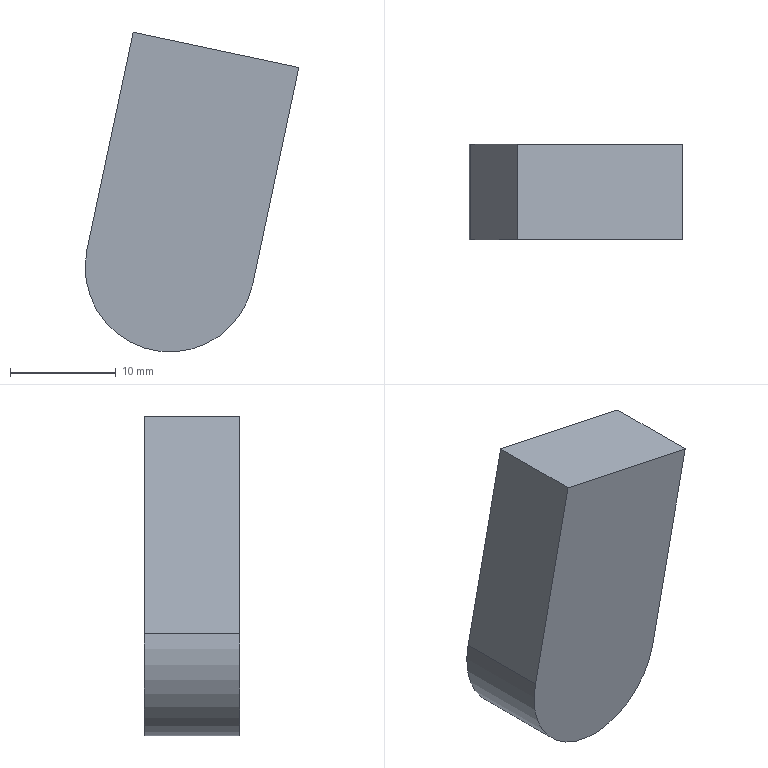Part | STEP file | HL4GZ-1.862.556 (flat key) 16×10×30 | 1 solid | 6 faces | box 20.191 x 9 x 30.204 mm | volume 3929 mm3 | plane 5 | cylinder 1 | commonest cylinder face diameters 16 x1
STEP:
#1=CARTESIAN_POINT('',(0.,0.,0.));
#2=DIRECTION('',(0.,0.,1.));
#3=DIRECTION('',(1.,0.,0.));
#4=AXIS2_PLACEMENT_3D('',#1,#2,#3);
#5=CARTESIAN_POINT('',(1970.277,-30.5,-346.911));
#6=VERTEX_POINT('',#5);
#7=CARTESIAN_POINT('',(1965.91,-30.5,-367.452));
#8=VERTEX_POINT('',#7);
#9=CARTESIAN_POINT('',(1967.314,-30.5,-360.85));
#10=DIRECTION('',(-0.2079,0.,-0.9781));
#11=VECTOR('',#10,1.);
#12=LINE('',#9,#11);
#13=CARTESIAN_POINT('',(1974.671,-30.5,-364.714));
#14=DIRECTION('',(0.,1.,0.));
#15=DIRECTION('',(-0.2079,0.,-0.9781));
#16=AXIS2_PLACEMENT_3D('',#13,#14,#15);
#17=PLANE('',#16);
#18=CARTESIAN_POINT('',(-2.25,8.));
#19=DIRECTION('',(1.,0.));
#20=VECTOR('',#19,1.);
#21=LINE('',#18,#20);
#22=(GEOMETRIC_REPRESENTATION_CONTEXT(2)PARAMETRIC_REPRESENTATION_CONTEXT()REPRESENTATION_CONTEXT('',''));
#23=DEFINITIONAL_REPRESENTATION('',(#21),#22);
#24=PCURVE('',#17,#23);
#25=CARTESIAN_POINT('',(1967.782,-21.5,-358.649));
#26=DIRECTION('',(-0.9781,0.,0.2079));
#27=DIRECTION('',(-0.2079,0.,-0.9781));
#28=AXIS2_PLACEMENT_3D('',#25,#26,#27);
#29=PLANE('',#28);
#30=CARTESIAN_POINT('',(2.25,9.));
#31=DIRECTION('',(1.,0.));
#32=VECTOR('',#31,1.);
#33=LINE('',#30,#32);
#34=(GEOMETRIC_REPRESENTATION_CONTEXT(2)PARAMETRIC_REPRESENTATION_CONTEXT()REPRESENTATION_CONTEXT('',''));
#35=DEFINITIONAL_REPRESENTATION('',(#33),#34);
#36=PCURVE('',#29,#35);
#37=SURFACE_CURVE('',#12,(#24,#36),.PCURVE_S1.);
#38=EDGE_CURVE('',#6,#8,#37,.T.);
#39=ORIENTED_EDGE('',*,*,#38,.T.);
#40=CARTESIAN_POINT('',(1981.561,-30.5,-370.779));
#41=VERTEX_POINT('',#40);
#42=CARTESIAN_POINT('',(1973.736,-30.5,-369.116));
#43=DIRECTION('',(0.,-1.,0.));
#44=DIRECTION('',(-0.9781,0.,0.2079));
#45=AXIS2_PLACEMENT_3D('',#42,#43,#44);
#46=CIRCLE('',#45,8.);
#47=CARTESIAN_POINT('',(4.5,8.));
#48=CARTESIAN_POINT('',(18.356,8.));
#49=CARTESIAN_POINT('',(11.428,-4.));
#50=CARTESIAN_POINT('',(4.5,-16.));
#51=CARTESIAN_POINT('',(-2.428,-4.));
#52=CARTESIAN_POINT('',(-9.356,8.));
#53=CARTESIAN_POINT('',(4.5,8.));
#54=(BOUNDED_CURVE()B_SPLINE_CURVE(2,(#47,#48,#49,#50,#51,#52,#53),.UNSPECIFIED.,.T.,.F.)B_SPLINE_CURVE_WITH_KNOTS((1,2,2,2,2,1),(-2.094,0.,2.094,4.189,6.283,8.378),.UNSPECIFIED.)CURVE()GEOMETRIC_REPRESENTATION_ITEM()RATIONAL_B_SPLINE_CURVE((1.,0.5,1.,0.5,1.,0.5,1.))REPRESENTATION_ITEM(''));
#55=(GEOMETRIC_REPRESENTATION_CONTEXT(2)PARAMETRIC_REPRESENTATION_CONTEXT()REPRESENTATION_CONTEXT('',''));
#56=DEFINITIONAL_REPRESENTATION('',(#54),#55);
#57=PCURVE('',#17,#56);
#58=CARTESIAN_POINT('',(1973.736,-21.5,-369.116));
#59=DIRECTION('',(0.,-1.,0.));
#60=DIRECTION('',(-0.9781,0.,0.2079));
#61=AXIS2_PLACEMENT_3D('',#58,#59,#60);
#62=CYLINDRICAL_SURFACE('',#61,8.);
#63=CARTESIAN_POINT('',(0.,9.));
#64=DIRECTION('',(1.,0.));
#65=VECTOR('',#64,1.);
#66=LINE('',#63,#65);
#67=(GEOMETRIC_REPRESENTATION_CONTEXT(2)PARAMETRIC_REPRESENTATION_CONTEXT()REPRESENTATION_CONTEXT('',''));
#68=DEFINITIONAL_REPRESENTATION('',(#66),#67);
#69=PCURVE('',#62,#68);
#70=SURFACE_CURVE('',#46,(#57,#69),.PCURVE_S1.);
#71=EDGE_CURVE('',#8,#41,#70,.T.);
#72=ORIENTED_EDGE('',*,*,#71,.T.);
#73=CARTESIAN_POINT('',(1985.927,-30.5,-350.238));
#74=VERTEX_POINT('',#73);
#75=CARTESIAN_POINT('',(1982.029,-30.5,-368.578));
#76=DIRECTION('',(0.2079,0.,0.9781));
#77=VECTOR('',#76,1.);
#78=LINE('',#75,#77);
#79=CARTESIAN_POINT('',(2.25,-8.));
#80=DIRECTION('',(-1.,0.));
#81=VECTOR('',#80,1.);
#82=LINE('',#79,#81);
#83=(GEOMETRIC_REPRESENTATION_CONTEXT(2)PARAMETRIC_REPRESENTATION_CONTEXT()REPRESENTATION_CONTEXT('',''));
#84=DEFINITIONAL_REPRESENTATION('',(#82),#83);
#85=PCURVE('',#17,#84);
#86=CARTESIAN_POINT('',(1981.561,-21.5,-370.779));
#87=DIRECTION('',(0.9781,0.,-0.2079));
#88=DIRECTION('',(0.2079,0.,0.9781));
#89=AXIS2_PLACEMENT_3D('',#86,#87,#88);
#90=PLANE('',#89);
#91=CARTESIAN_POINT('',(2.25,9.));
#92=DIRECTION('',(1.,0.));
#93=VECTOR('',#92,1.);
#94=LINE('',#91,#93);
#95=(GEOMETRIC_REPRESENTATION_CONTEXT(2)PARAMETRIC_REPRESENTATION_CONTEXT()REPRESENTATION_CONTEXT('',''));
#96=DEFINITIONAL_REPRESENTATION('',(#94),#95);
#97=PCURVE('',#90,#96);
#98=SURFACE_CURVE('',#78,(#85,#97),.PCURVE_S1.);
#99=EDGE_CURVE('',#41,#74,#98,.T.);
#100=ORIENTED_EDGE('',*,*,#99,.T.);
#101=CARTESIAN_POINT('',(1971.255,-30.5,-347.119));
#102=DIRECTION('',(-0.9781,0.,0.2079));
#103=VECTOR('',#102,1.);
#104=LINE('',#101,#103);
#105=CARTESIAN_POINT('',(-16.5,7.));
#106=DIRECTION('',(0.,1.));
#107=VECTOR('',#106,1.);
#108=LINE('',#105,#107);
#109=(GEOMETRIC_REPRESENTATION_CONTEXT(2)PARAMETRIC_REPRESENTATION_CONTEXT()REPRESENTATION_CONTEXT('',''));
#110=DEFINITIONAL_REPRESENTATION('',(#108),#109);
#111=PCURVE('',#17,#110);
#112=CARTESIAN_POINT('',(1984.949,-21.5,-350.03));
#113=DIRECTION('',(0.2079,0.,0.9781));
#114=DIRECTION('',(-0.9781,0.,0.2079));
#115=AXIS2_PLACEMENT_3D('',#112,#113,#114);
#116=PLANE('',#115);
#117=CARTESIAN_POINT('',(14.,9.));
#118=DIRECTION('',(1.,0.));
#119=VECTOR('',#118,1.);
#120=LINE('',#117,#119);
#121=(GEOMETRIC_REPRESENTATION_CONTEXT(2)PARAMETRIC_REPRESENTATION_CONTEXT()REPRESENTATION_CONTEXT('',''));
#122=DEFINITIONAL_REPRESENTATION('',(#120),#121);
#123=PCURVE('',#116,#122);
#124=SURFACE_CURVE('',#104,(#111,#123),.PCURVE_S1.);
#125=EDGE_CURVE('',#74,#6,#124,.T.);
#126=ORIENTED_EDGE('',*,*,#125,.T.);
#127=EDGE_LOOP('',(#39,#72,#100,#126));
#128=FACE_BOUND('',#127,.T.);
#129=ADVANCED_FACE('',(#128),#17,.F.);
#130=CARTESIAN_POINT('',(1965.91,-21.5,-367.452));
#131=VERTEX_POINT('',#130);
#132=CARTESIAN_POINT('',(1981.561,-21.5,-370.779));
#133=VERTEX_POINT('',#132);
#134=CARTESIAN_POINT('',(1973.736,-21.5,-369.116));
#135=DIRECTION('',(0.,-1.,0.));
#136=DIRECTION('',(-0.9781,0.,0.2079));
#137=AXIS2_PLACEMENT_3D('',#134,#135,#136);
#138=CIRCLE('',#137,8.);
#139=CARTESIAN_POINT('',(0.,0.));
#140=DIRECTION('',(1.,0.));
#141=VECTOR('',#140,1.);
#142=LINE('',#139,#141);
#143=(GEOMETRIC_REPRESENTATION_CONTEXT(2)PARAMETRIC_REPRESENTATION_CONTEXT()REPRESENTATION_CONTEXT('',''));
#144=DEFINITIONAL_REPRESENTATION('',(#142),#143);
#145=PCURVE('',#62,#144);
#146=CARTESIAN_POINT('',(1974.671,-21.5,-364.714));
#147=DIRECTION('',(0.,1.,0.));
#148=DIRECTION('',(-0.2079,0.,-0.9781));
#149=AXIS2_PLACEMENT_3D('',#146,#147,#148);
#150=PLANE('',#149);
#151=CARTESIAN_POINT('',(4.5,8.));
#152=CARTESIAN_POINT('',(18.356,8.));
#153=CARTESIAN_POINT('',(11.428,-4.));
#154=CARTESIAN_POINT('',(4.5,-16.));
#155=CARTESIAN_POINT('',(-2.428,-4.));
#156=CARTESIAN_POINT('',(-9.356,8.));
#157=CARTESIAN_POINT('',(4.5,8.));
#158=(BOUNDED_CURVE()B_SPLINE_CURVE(2,(#151,#152,#153,#154,#155,#156,#157),.UNSPECIFIED.,.T.,.F.)B_SPLINE_CURVE_WITH_KNOTS((1,2,2,2,2,1),(-2.094,0.,2.094,4.189,6.283,8.378),.UNSPECIFIED.)CURVE()GEOMETRIC_REPRESENTATION_ITEM()RATIONAL_B_SPLINE_CURVE((1.,0.5,1.,0.5,1.,0.5,1.))REPRESENTATION_ITEM(''));
#159=(GEOMETRIC_REPRESENTATION_CONTEXT(2)PARAMETRIC_REPRESENTATION_CONTEXT()REPRESENTATION_CONTEXT('',''));
#160=DEFINITIONAL_REPRESENTATION('',(#158),#159);
#161=PCURVE('',#150,#160);
#162=SURFACE_CURVE('',#138,(#145,#161),.PCURVE_S1.);
#163=EDGE_CURVE('',#131,#133,#162,.T.);
#164=ORIENTED_EDGE('',*,*,#163,.T.);
#165=CARTESIAN_POINT('',(1981.561,-21.5,-370.779));
#166=DIRECTION('',(0.,-1.,0.));
#167=VECTOR('',#166,1.);
#168=LINE('',#165,#167);
#169=CARTESIAN_POINT('',(3.142,0.));
#170=DIRECTION('',(0.,1.));
#171=VECTOR('',#170,1.);
#172=LINE('',#169,#171);
#173=(GEOMETRIC_REPRESENTATION_CONTEXT(2)PARAMETRIC_REPRESENTATION_CONTEXT()REPRESENTATION_CONTEXT('',''));
#174=DEFINITIONAL_REPRESENTATION('',(#172),#173);
#175=PCURVE('',#62,#174);
#176=CARTESIAN_POINT('',(0.,0.));
#177=DIRECTION('',(0.,1.));
#178=VECTOR('',#177,1.);
#179=LINE('',#176,#178);
#180=(GEOMETRIC_REPRESENTATION_CONTEXT(2)PARAMETRIC_REPRESENTATION_CONTEXT()REPRESENTATION_CONTEXT('',''));
#181=DEFINITIONAL_REPRESENTATION('',(#179),#180);
#182=PCURVE('',#90,#181);
#183=SURFACE_CURVE('',#168,(#175,#182),.PCURVE_S1.);
#184=EDGE_CURVE('',#133,#41,#183,.T.);
#185=ORIENTED_EDGE('',*,*,#184,.T.);
#186=ORIENTED_EDGE('',*,*,#71,.F.);
#187=CARTESIAN_POINT('',(1965.91,-21.5,-367.452));
#188=DIRECTION('',(0.,-1.,0.));
#189=VECTOR('',#188,1.);
#190=LINE('',#187,#189);
#191=CARTESIAN_POINT('',(0.,0.));
#192=DIRECTION('',(0.,1.));
#193=VECTOR('',#192,1.);
#194=LINE('',#191,#193);
#195=(GEOMETRIC_REPRESENTATION_CONTEXT(2)PARAMETRIC_REPRESENTATION_CONTEXT()REPRESENTATION_CONTEXT('',''));
#196=DEFINITIONAL_REPRESENTATION('',(#194),#195);
#197=PCURVE('',#62,#196);
#198=CARTESIAN_POINT('',(9.,0.));
#199=DIRECTION('',(0.,1.));
#200=VECTOR('',#199,1.);
#201=LINE('',#198,#200);
#202=(GEOMETRIC_REPRESENTATION_CONTEXT(2)PARAMETRIC_REPRESENTATION_CONTEXT()REPRESENTATION_CONTEXT('',''));
#203=DEFINITIONAL_REPRESENTATION('',(#201),#202);
#204=PCURVE('',#29,#203);
#205=SURFACE_CURVE('',#190,(#197,#204),.PCURVE_S1.);
#206=EDGE_CURVE('',#131,#8,#205,.T.);
#207=ORIENTED_EDGE('',*,*,#206,.F.);
#208=EDGE_LOOP('',(#164,#185,#186,#207));
#209=FACE_BOUND('',#208,.T.);
#210=ADVANCED_FACE('',(#209),#62,.T.);
#211=ORIENTED_EDGE('',*,*,#99,.F.);
#212=ORIENTED_EDGE('',*,*,#184,.F.);
#213=CARTESIAN_POINT('',(1985.927,-21.5,-350.238));
#214=VERTEX_POINT('',#213);
#215=CARTESIAN_POINT('',(1982.029,-21.5,-368.578));
#216=DIRECTION('',(0.2079,0.,0.9781));
#217=VECTOR('',#216,1.);
#218=LINE('',#215,#217);
#219=CARTESIAN_POINT('',(2.25,0.));
#220=DIRECTION('',(1.,0.));
#221=VECTOR('',#220,1.);
#222=LINE('',#219,#221);
#223=(GEOMETRIC_REPRESENTATION_CONTEXT(2)PARAMETRIC_REPRESENTATION_CONTEXT()REPRESENTATION_CONTEXT('',''));
#224=DEFINITIONAL_REPRESENTATION('',(#222),#223);
#225=PCURVE('',#90,#224);
#226=CARTESIAN_POINT('',(2.25,-8.));
#227=DIRECTION('',(-1.,0.));
#228=VECTOR('',#227,1.);
#229=LINE('',#226,#228);
#230=(GEOMETRIC_REPRESENTATION_CONTEXT(2)PARAMETRIC_REPRESENTATION_CONTEXT()REPRESENTATION_CONTEXT('',''));
#231=DEFINITIONAL_REPRESENTATION('',(#229),#230);
#232=PCURVE('',#150,#231);
#233=SURFACE_CURVE('',#218,(#225,#232),.PCURVE_S1.);
#234=EDGE_CURVE('',#133,#214,#233,.T.);
#235=ORIENTED_EDGE('',*,*,#234,.T.);
#236=CARTESIAN_POINT('',(1985.927,-21.5,-350.238));
#237=DIRECTION('',(0.,-1.,0.));
#238=VECTOR('',#237,1.);
#239=LINE('',#236,#238);
#240=CARTESIAN_POINT('',(21.,0.));
#241=DIRECTION('',(0.,1.));
#242=VECTOR('',#241,1.);
#243=LINE('',#240,#242);
#244=(GEOMETRIC_REPRESENTATION_CONTEXT(2)PARAMETRIC_REPRESENTATION_CONTEXT()REPRESENTATION_CONTEXT('',''));
#245=DEFINITIONAL_REPRESENTATION('',(#243),#244);
#246=PCURVE('',#90,#245);
#247=CARTESIAN_POINT('',(-1.,0.));
#248=DIRECTION('',(0.,1.));
#249=VECTOR('',#248,1.);
#250=LINE('',#247,#249);
#251=(GEOMETRIC_REPRESENTATION_CONTEXT(2)PARAMETRIC_REPRESENTATION_CONTEXT()REPRESENTATION_CONTEXT('',''));
#252=DEFINITIONAL_REPRESENTATION('',(#250),#251);
#253=PCURVE('',#116,#252);
#254=SURFACE_CURVE('',#239,(#246,#253),.PCURVE_S1.);
#255=EDGE_CURVE('',#214,#74,#254,.T.);
#256=ORIENTED_EDGE('',*,*,#255,.T.);
#257=EDGE_LOOP('',(#211,#212,#235,#256));
#258=FACE_BOUND('',#257,.T.);
#259=ADVANCED_FACE('',(#258),#90,.T.);
#260=ORIENTED_EDGE('',*,*,#234,.F.);
#261=ORIENTED_EDGE('',*,*,#163,.F.);
#262=CARTESIAN_POINT('',(1970.277,-21.5,-346.911));
#263=VERTEX_POINT('',#262);
#264=CARTESIAN_POINT('',(1967.314,-21.5,-360.85));
#265=DIRECTION('',(-0.2079,0.,-0.9781));
#266=VECTOR('',#265,1.);
#267=LINE('',#264,#266);
#268=CARTESIAN_POINT('',(-2.25,8.));
#269=DIRECTION('',(1.,0.));
#270=VECTOR('',#269,1.);
#271=LINE('',#268,#270);
#272=(GEOMETRIC_REPRESENTATION_CONTEXT(2)PARAMETRIC_REPRESENTATION_CONTEXT()REPRESENTATION_CONTEXT('',''));
#273=DEFINITIONAL_REPRESENTATION('',(#271),#272);
#274=PCURVE('',#150,#273);
#275=CARTESIAN_POINT('',(2.25,0.));
#276=DIRECTION('',(1.,0.));
#277=VECTOR('',#276,1.);
#278=LINE('',#275,#277);
#279=(GEOMETRIC_REPRESENTATION_CONTEXT(2)PARAMETRIC_REPRESENTATION_CONTEXT()REPRESENTATION_CONTEXT('',''));
#280=DEFINITIONAL_REPRESENTATION('',(#278),#279);
#281=PCURVE('',#29,#280);
#282=SURFACE_CURVE('',#267,(#274,#281),.PCURVE_S1.);
#283=EDGE_CURVE('',#263,#131,#282,.T.);
#284=ORIENTED_EDGE('',*,*,#283,.F.);
#285=CARTESIAN_POINT('',(1971.255,-21.5,-347.119));
#286=DIRECTION('',(0.9781,0.,-0.2079));
#287=VECTOR('',#286,1.);
#288=LINE('',#285,#287);
#289=CARTESIAN_POINT('',(-16.5,7.));
#290=DIRECTION('',(0.,-1.));
#291=VECTOR('',#290,1.);
#292=LINE('',#289,#291);
#293=(GEOMETRIC_REPRESENTATION_CONTEXT(2)PARAMETRIC_REPRESENTATION_CONTEXT()REPRESENTATION_CONTEXT('',''));
#294=DEFINITIONAL_REPRESENTATION('',(#292),#293);
#295=PCURVE('',#150,#294);
#296=CARTESIAN_POINT('',(14.,0.));
#297=DIRECTION('',(-1.,0.));
#298=VECTOR('',#297,1.);
#299=LINE('',#296,#298);
#300=(GEOMETRIC_REPRESENTATION_CONTEXT(2)PARAMETRIC_REPRESENTATION_CONTEXT()REPRESENTATION_CONTEXT('',''));
#301=DEFINITIONAL_REPRESENTATION('',(#299),#300);
#302=PCURVE('',#116,#301);
#303=SURFACE_CURVE('',#288,(#295,#302),.PCURVE_S1.);
#304=EDGE_CURVE('',#263,#214,#303,.T.);
#305=ORIENTED_EDGE('',*,*,#304,.T.);
#306=EDGE_LOOP('',(#260,#261,#284,#305));
#307=FACE_BOUND('',#306,.T.);
#308=ADVANCED_FACE('',(#307),#150,.T.);
#309=ORIENTED_EDGE('',*,*,#283,.T.);
#310=ORIENTED_EDGE('',*,*,#206,.T.);
#311=ORIENTED_EDGE('',*,*,#38,.F.);
#312=CARTESIAN_POINT('',(1970.277,-21.5,-346.911));
#313=DIRECTION('',(0.,-1.,0.));
#314=VECTOR('',#313,1.);
#315=LINE('',#312,#314);
#316=CARTESIAN_POINT('',(-12.,0.));
#317=DIRECTION('',(0.,1.));
#318=VECTOR('',#317,1.);
#319=LINE('',#316,#318);
#320=(GEOMETRIC_REPRESENTATION_CONTEXT(2)PARAMETRIC_REPRESENTATION_CONTEXT()REPRESENTATION_CONTEXT('',''));
#321=DEFINITIONAL_REPRESENTATION('',(#319),#320);
#322=PCURVE('',#29,#321);
#323=CARTESIAN_POINT('',(15.,0.));
#324=DIRECTION('',(0.,1.));
#325=VECTOR('',#324,1.);
#326=LINE('',#323,#325);
#327=(GEOMETRIC_REPRESENTATION_CONTEXT(2)PARAMETRIC_REPRESENTATION_CONTEXT()REPRESENTATION_CONTEXT('',''));
#328=DEFINITIONAL_REPRESENTATION('',(#326),#327);
#329=PCURVE('',#116,#328);
#330=SURFACE_CURVE('',#315,(#322,#329),.PCURVE_S1.);
#331=EDGE_CURVE('',#263,#6,#330,.T.);
#332=ORIENTED_EDGE('',*,*,#331,.F.);
#333=EDGE_LOOP('',(#309,#310,#311,#332));
#334=FACE_BOUND('',#333,.T.);
#335=ADVANCED_FACE('',(#334),#29,.T.);
#336=ORIENTED_EDGE('',*,*,#304,.F.);
#337=ORIENTED_EDGE('',*,*,#331,.T.);
#338=ORIENTED_EDGE('',*,*,#125,.F.);
#339=ORIENTED_EDGE('',*,*,#255,.F.);
#340=EDGE_LOOP('',(#336,#337,#338,#339));
#341=FACE_BOUND('',#340,.T.);
#342=ADVANCED_FACE('',(#341),#116,.T.);
#343=CLOSED_SHELL('',(#129,#210,#259,#308,#335,#342));
#344=MANIFOLD_SOLID_BREP('',#343);
#345=(LENGTH_UNIT()NAMED_UNIT(*)SI_UNIT(.MILLI.,.METRE.));
#346=UNCERTAINTY_MEASURE_WITH_UNIT(LENGTH_MEASURE(0.0000001),#345,'','');
#347=(NAMED_UNIT(*)PLANE_ANGLE_UNIT()SI_UNIT($,.RADIAN.));
#348=(NAMED_UNIT(*)SI_UNIT($,.STERADIAN.)SOLID_ANGLE_UNIT());
#349=(GEOMETRIC_REPRESENTATION_CONTEXT(3)GLOBAL_UNCERTAINTY_ASSIGNED_CONTEXT((#346))GLOBAL_UNIT_ASSIGNED_CONTEXT((#345,#347,#348))REPRESENTATION_CONTEXT('',''));
#350=ADVANCED_BREP_SHAPE_REPRESENTATION('',(#4,#344),#349);